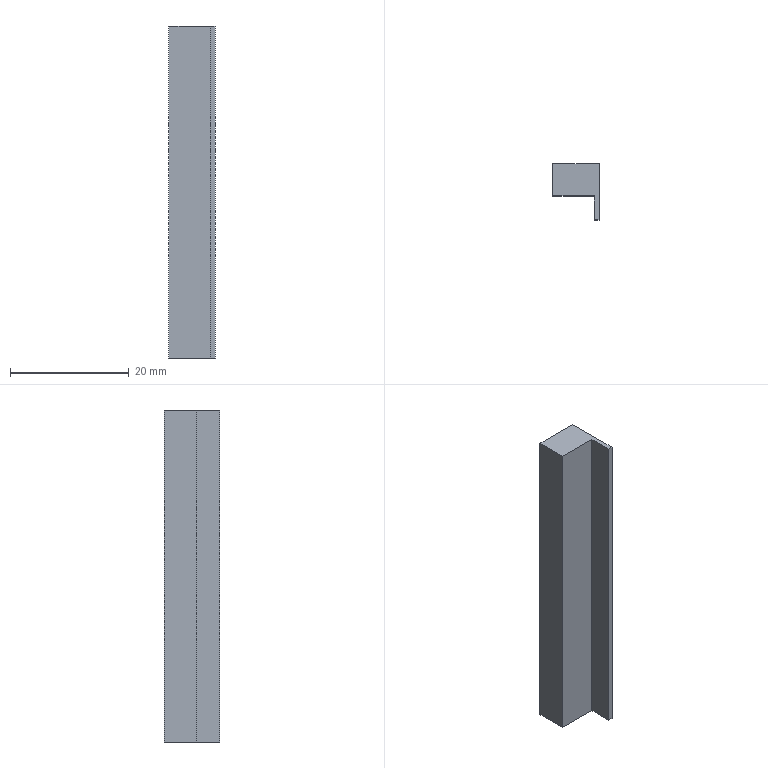Part | NX | features BREP 2 | 2 solids | 16 faces | box 7.8 x 9.398 x 56 mm | volume 5074 mm3 | plane 16
STEP:
#1=CARTESIAN_POINT('',(3.9,4.699,-4.));
#2=VERTEX_POINT('',#1);
#3=CARTESIAN_POINT('',(3.9,4.699,52.));
#4=VERTEX_POINT('',#3);
#5=CARTESIAN_POINT('',(3.9,4.699,0.));
#6=DIRECTION('',(0.,0.,1.));
#7=VECTOR('',#6,1000.);
#8=LINE('',#5,#7);
#9=EDGE_CURVE('',#2,#4,#8,.T.);
#10=ORIENTED_EDGE('',*,*,#9,.T.);
#11=CARTESIAN_POINT('',(3.9,-4.699,52.));
#12=VERTEX_POINT('',#11);
#13=CARTESIAN_POINT('',(3.9,-26.301,52.));
#14=DIRECTION('',(0.,1.,0.));
#15=VECTOR('',#14,1000.);
#16=LINE('',#13,#15);
#17=EDGE_CURVE('',#12,#4,#16,.T.);
#18=ORIENTED_EDGE('',*,*,#17,.F.);
#19=CARTESIAN_POINT('',(3.9,-4.699,-4.));
#20=VERTEX_POINT('',#19);
#21=CARTESIAN_POINT('',(3.9,-4.699,0.));
#22=DIRECTION('',(0.,0.,1.));
#23=VECTOR('',#22,1000.);
#24=LINE('',#21,#23);
#25=EDGE_CURVE('',#20,#12,#24,.T.);
#26=ORIENTED_EDGE('',*,*,#25,.F.);
#27=CARTESIAN_POINT('',(3.9,-26.301,-4.));
#28=DIRECTION('',(0.,1.,0.));
#29=VECTOR('',#28,1000.);
#30=LINE('',#27,#29);
#31=EDGE_CURVE('',#20,#2,#30,.T.);
#32=ORIENTED_EDGE('',*,*,#31,.T.);
#33=EDGE_LOOP('',(#10,#18,#26,#32));
#34=FACE_BOUND('',#33,.T.);
#35=CARTESIAN_POINT('',(3.9,4.699,0.));
#36=DIRECTION('',(-1.,0.,0.));
#37=DIRECTION('',(0.,1.,0.));
#38=AXIS2_PLACEMENT_3D('',#35,#36,#37);
#39=PLANE('',#38);
#40=ADVANCED_FACE('',(#34),#39,.F.);
#41=ORIENTED_EDGE('',*,*,#25,.T.);
#42=CARTESIAN_POINT('',(3.1,-4.699,52.));
#43=VERTEX_POINT('',#42);
#44=CARTESIAN_POINT('',(-9.65,-4.699,52.));
#45=DIRECTION('',(1.,0.,0.));
#46=VECTOR('',#45,1000.);
#47=LINE('',#44,#46);
#48=EDGE_CURVE('',#43,#12,#47,.T.);
#49=ORIENTED_EDGE('',*,*,#48,.F.);
#50=CARTESIAN_POINT('',(3.1,-4.699,-4.));
#51=VERTEX_POINT('',#50);
#52=CARTESIAN_POINT('',(3.1,-4.699,0.));
#53=DIRECTION('',(0.,0.,1.));
#54=VECTOR('',#53,1000.);
#55=LINE('',#52,#54);
#56=EDGE_CURVE('',#51,#43,#55,.T.);
#57=ORIENTED_EDGE('',*,*,#56,.F.);
#58=CARTESIAN_POINT('',(-9.65,-4.699,-4.));
#59=DIRECTION('',(1.,0.,0.));
#60=VECTOR('',#59,1000.);
#61=LINE('',#58,#60);
#62=EDGE_CURVE('',#51,#20,#61,.T.);
#63=ORIENTED_EDGE('',*,*,#62,.T.);
#64=EDGE_LOOP('',(#41,#49,#57,#63));
#65=FACE_BOUND('',#64,.T.);
#66=CARTESIAN_POINT('',(3.9,-4.699,0.));
#67=DIRECTION('',(0.,1.,0.));
#68=DIRECTION('',(1.,0.,0.));
#69=AXIS2_PLACEMENT_3D('',#66,#67,#68);
#70=PLANE('',#69);
#71=ADVANCED_FACE('',(#65),#70,.F.);
#72=ORIENTED_EDGE('',*,*,#56,.T.);
#73=CARTESIAN_POINT('',(3.1,-0.6992,52.));
#74=VERTEX_POINT('',#73);
#75=CARTESIAN_POINT('',(3.1,-26.301,52.));
#76=DIRECTION('',(0.,-1.,0.));
#77=VECTOR('',#76,1000.);
#78=LINE('',#75,#77);
#79=EDGE_CURVE('',#74,#43,#78,.T.);
#80=ORIENTED_EDGE('',*,*,#79,.F.);
#81=CARTESIAN_POINT('',(3.1,-0.6992,-4.));
#82=VERTEX_POINT('',#81);
#83=CARTESIAN_POINT('',(3.1,-0.6992,0.));
#84=DIRECTION('',(0.,0.,1.));
#85=VECTOR('',#84,1000.);
#86=LINE('',#83,#85);
#87=EDGE_CURVE('',#82,#74,#86,.T.);
#88=ORIENTED_EDGE('',*,*,#87,.F.);
#89=CARTESIAN_POINT('',(3.1,-26.301,-4.));
#90=DIRECTION('',(0.,-1.,0.));
#91=VECTOR('',#90,1000.);
#92=LINE('',#89,#91);
#93=EDGE_CURVE('',#82,#51,#92,.T.);
#94=ORIENTED_EDGE('',*,*,#93,.T.);
#95=EDGE_LOOP('',(#72,#80,#88,#94));
#96=FACE_BOUND('',#95,.T.);
#97=CARTESIAN_POINT('',(3.1,-4.699,0.));
#98=DIRECTION('',(1.,0.,0.));
#99=DIRECTION('',(0.,-1.,0.));
#100=AXIS2_PLACEMENT_3D('',#97,#98,#99);
#101=PLANE('',#100);
#102=ADVANCED_FACE('',(#96),#101,.F.);
#103=ORIENTED_EDGE('',*,*,#87,.T.);
#104=CARTESIAN_POINT('',(-3.9,-0.6992,52.));
#105=VERTEX_POINT('',#104);
#106=CARTESIAN_POINT('',(-9.65,-0.6992,52.));
#107=DIRECTION('',(1.,0.,0.));
#108=VECTOR('',#107,1000.);
#109=LINE('',#106,#108);
#110=EDGE_CURVE('',#105,#74,#109,.T.);
#111=ORIENTED_EDGE('',*,*,#110,.F.);
#112=CARTESIAN_POINT('',(-3.9,-0.6992,-4.));
#113=VERTEX_POINT('',#112);
#114=CARTESIAN_POINT('',(-3.9,-0.6992,0.));
#115=DIRECTION('',(0.,0.,1.));
#116=VECTOR('',#115,1000.);
#117=LINE('',#114,#116);
#118=EDGE_CURVE('',#113,#105,#117,.T.);
#119=ORIENTED_EDGE('',*,*,#118,.F.);
#120=CARTESIAN_POINT('',(-9.65,-0.6992,-4.));
#121=DIRECTION('',(1.,0.,0.));
#122=VECTOR('',#121,1000.);
#123=LINE('',#120,#122);
#124=EDGE_CURVE('',#113,#82,#123,.T.);
#125=ORIENTED_EDGE('',*,*,#124,.T.);
#126=EDGE_LOOP('',(#103,#111,#119,#125));
#127=FACE_BOUND('',#126,.T.);
#128=CARTESIAN_POINT('',(3.1,-0.6992,0.));
#129=DIRECTION('',(0.,1.,0.));
#130=DIRECTION('',(1.,0.,0.));
#131=AXIS2_PLACEMENT_3D('',#128,#129,#130);
#132=PLANE('',#131);
#133=ADVANCED_FACE('',(#127),#132,.F.);
#134=CARTESIAN_POINT('',(-3.9,4.699,-4.));
#135=VERTEX_POINT('',#134);
#136=CARTESIAN_POINT('',(-3.9,4.699,52.));
#137=VERTEX_POINT('',#136);
#138=CARTESIAN_POINT('',(-3.9,4.699,0.));
#139=DIRECTION('',(0.,0.,1.));
#140=VECTOR('',#139,1000.);
#141=LINE('',#138,#140);
#142=EDGE_CURVE('',#135,#137,#141,.T.);
#143=ORIENTED_EDGE('',*,*,#142,.F.);
#144=CARTESIAN_POINT('',(-3.9,-26.301,-4.));
#145=DIRECTION('',(0.,-1.,0.));
#146=VECTOR('',#145,1000.);
#147=LINE('',#144,#146);
#148=EDGE_CURVE('',#135,#113,#147,.T.);
#149=ORIENTED_EDGE('',*,*,#148,.T.);
#150=ORIENTED_EDGE('',*,*,#118,.T.);
#151=CARTESIAN_POINT('',(-3.9,-26.301,52.));
#152=DIRECTION('',(0.,-1.,0.));
#153=VECTOR('',#152,1000.);
#154=LINE('',#151,#153);
#155=EDGE_CURVE('',#137,#105,#154,.T.);
#156=ORIENTED_EDGE('',*,*,#155,.F.);
#157=EDGE_LOOP('',(#143,#149,#150,#156));
#158=FACE_BOUND('',#157,.T.);
#159=CARTESIAN_POINT('',(-3.9,2.201,0.));
#160=DIRECTION('',(1.,0.,0.));
#161=DIRECTION('',(0.,-1.,0.));
#162=AXIS2_PLACEMENT_3D('',#159,#160,#161);
#163=PLANE('',#162);
#164=ADVANCED_FACE('',(#158),#163,.F.);
#165=CARTESIAN_POINT('',(-9.65,4.699,-4.));
#166=DIRECTION('',(-1.,0.,0.));
#167=VECTOR('',#166,1000.);
#168=LINE('',#165,#167);
#169=EDGE_CURVE('',#2,#135,#168,.T.);
#170=ORIENTED_EDGE('',*,*,#169,.T.);
#171=ORIENTED_EDGE('',*,*,#142,.T.);
#172=CARTESIAN_POINT('',(-9.65,4.699,52.));
#173=DIRECTION('',(-1.,0.,0.));
#174=VECTOR('',#173,1000.);
#175=LINE('',#172,#174);
#176=EDGE_CURVE('',#4,#137,#175,.T.);
#177=ORIENTED_EDGE('',*,*,#176,.F.);
#178=ORIENTED_EDGE('',*,*,#9,.F.);
#179=EDGE_LOOP('',(#170,#171,#177,#178));
#180=FACE_BOUND('',#179,.T.);
#181=CARTESIAN_POINT('',(-3.9,4.699,0.));
#182=DIRECTION('',(0.,-1.,0.));
#183=DIRECTION('',(-1.,0.,0.));
#184=AXIS2_PLACEMENT_3D('',#181,#182,#183);
#185=PLANE('',#184);
#186=ADVANCED_FACE('',(#180),#185,.F.);
#187=ORIENTED_EDGE('',*,*,#155,.T.);
#188=ORIENTED_EDGE('',*,*,#110,.T.);
#189=ORIENTED_EDGE('',*,*,#79,.T.);
#190=ORIENTED_EDGE('',*,*,#48,.T.);
#191=ORIENTED_EDGE('',*,*,#17,.T.);
#192=ORIENTED_EDGE('',*,*,#176,.T.);
#193=EDGE_LOOP('',(#187,#188,#189,#190,#191,#192));
#194=FACE_BOUND('',#193,.T.);
#195=CARTESIAN_POINT('',(-9.65,-26.301,52.));
#196=DIRECTION('',(0.,0.,1.));
#197=DIRECTION('',(-1.,0.,0.));
#198=AXIS2_PLACEMENT_3D('',#195,#196,#197);
#199=PLANE('',#198);
#200=ADVANCED_FACE('',(#194),#199,.T.);
#201=ORIENTED_EDGE('',*,*,#148,.F.);
#202=ORIENTED_EDGE('',*,*,#169,.F.);
#203=ORIENTED_EDGE('',*,*,#31,.F.);
#204=ORIENTED_EDGE('',*,*,#62,.F.);
#205=ORIENTED_EDGE('',*,*,#93,.F.);
#206=ORIENTED_EDGE('',*,*,#124,.F.);
#207=EDGE_LOOP('',(#201,#202,#203,#204,#205,#206));
#208=FACE_BOUND('',#207,.T.);
#209=CARTESIAN_POINT('',(-9.65,-26.301,-4.));
#210=DIRECTION('',(0.,0.,1.));
#211=DIRECTION('',(-1.,0.,0.));
#212=AXIS2_PLACEMENT_3D('',#209,#210,#211);
#213=PLANE('',#212);
#214=ADVANCED_FACE('',(#208),#213,.F.);
#215=CLOSED_SHELL('',(#40,#71,#102,#133,#164,#186,#200,#214));
#216=MANIFOLD_SOLID_BREP('',#215);
#217=CARTESIAN_POINT('',(3.9,4.699,-4.));
#218=VERTEX_POINT('',#217);
#219=CARTESIAN_POINT('',(3.9,4.699,52.));
#220=VERTEX_POINT('',#219);
#221=CARTESIAN_POINT('',(3.9,4.699,0.));
#222=DIRECTION('',(0.,0.,1.));
#223=VECTOR('',#222,1000.);
#224=LINE('',#221,#223);
#225=EDGE_CURVE('',#218,#220,#224,.T.);
#226=ORIENTED_EDGE('',*,*,#225,.T.);
#227=CARTESIAN_POINT('',(3.9,-4.699,52.));
#228=VERTEX_POINT('',#227);
#229=CARTESIAN_POINT('',(3.9,-26.301,52.));
#230=DIRECTION('',(0.,1.,0.));
#231=VECTOR('',#230,1000.);
#232=LINE('',#229,#231);
#233=EDGE_CURVE('',#228,#220,#232,.T.);
#234=ORIENTED_EDGE('',*,*,#233,.F.);
#235=CARTESIAN_POINT('',(3.9,-4.699,-4.));
#236=VERTEX_POINT('',#235);
#237=CARTESIAN_POINT('',(3.9,-4.699,0.));
#238=DIRECTION('',(0.,0.,1.));
#239=VECTOR('',#238,1000.);
#240=LINE('',#237,#239);
#241=EDGE_CURVE('',#236,#228,#240,.T.);
#242=ORIENTED_EDGE('',*,*,#241,.F.);
#243=CARTESIAN_POINT('',(3.9,-26.301,-4.));
#244=DIRECTION('',(0.,1.,0.));
#245=VECTOR('',#244,1000.);
#246=LINE('',#243,#245);
#247=EDGE_CURVE('',#236,#218,#246,.T.);
#248=ORIENTED_EDGE('',*,*,#247,.T.);
#249=EDGE_LOOP('',(#226,#234,#242,#248));
#250=FACE_BOUND('',#249,.T.);
#251=CARTESIAN_POINT('',(3.9,4.699,0.));
#252=DIRECTION('',(-1.,0.,0.));
#253=DIRECTION('',(0.,1.,0.));
#254=AXIS2_PLACEMENT_3D('',#251,#252,#253);
#255=PLANE('',#254);
#256=ADVANCED_FACE('',(#250),#255,.F.);
#257=ORIENTED_EDGE('',*,*,#241,.T.);
#258=CARTESIAN_POINT('',(3.1,-4.699,52.));
#259=VERTEX_POINT('',#258);
#260=CARTESIAN_POINT('',(-9.65,-4.699,52.));
#261=DIRECTION('',(1.,0.,0.));
#262=VECTOR('',#261,1000.);
#263=LINE('',#260,#262);
#264=EDGE_CURVE('',#259,#228,#263,.T.);
#265=ORIENTED_EDGE('',*,*,#264,.F.);
#266=CARTESIAN_POINT('',(3.1,-4.699,-4.));
#267=VERTEX_POINT('',#266);
#268=CARTESIAN_POINT('',(3.1,-4.699,0.));
#269=DIRECTION('',(0.,0.,1.));
#270=VECTOR('',#269,1000.);
#271=LINE('',#268,#270);
#272=EDGE_CURVE('',#267,#259,#271,.T.);
#273=ORIENTED_EDGE('',*,*,#272,.F.);
#274=CARTESIAN_POINT('',(-9.65,-4.699,-4.));
#275=DIRECTION('',(1.,0.,0.));
#276=VECTOR('',#275,1000.);
#277=LINE('',#274,#276);
#278=EDGE_CURVE('',#267,#236,#277,.T.);
#279=ORIENTED_EDGE('',*,*,#278,.T.);
#280=EDGE_LOOP('',(#257,#265,#273,#279));
#281=FACE_BOUND('',#280,.T.);
#282=CARTESIAN_POINT('',(3.9,-4.699,0.));
#283=DIRECTION('',(0.,1.,0.));
#284=DIRECTION('',(1.,0.,0.));
#285=AXIS2_PLACEMENT_3D('',#282,#283,#284);
#286=PLANE('',#285);
#287=ADVANCED_FACE('',(#281),#286,.F.);
#288=ORIENTED_EDGE('',*,*,#272,.T.);
#289=CARTESIAN_POINT('',(3.1,-0.6992,52.));
#290=VERTEX_POINT('',#289);
#291=CARTESIAN_POINT('',(3.1,-26.301,52.));
#292=DIRECTION('',(0.,-1.,0.));
#293=VECTOR('',#292,1000.);
#294=LINE('',#291,#293);
#295=EDGE_CURVE('',#290,#259,#294,.T.);
#296=ORIENTED_EDGE('',*,*,#295,.F.);
#297=CARTESIAN_POINT('',(3.1,-0.6992,-4.));
#298=VERTEX_POINT('',#297);
#299=CARTESIAN_POINT('',(3.1,-0.6992,0.));
#300=DIRECTION('',(0.,0.,1.));
#301=VECTOR('',#300,1000.);
#302=LINE('',#299,#301);
#303=EDGE_CURVE('',#298,#290,#302,.T.);
#304=ORIENTED_EDGE('',*,*,#303,.F.);
#305=CARTESIAN_POINT('',(3.1,-26.301,-4.));
#306=DIRECTION('',(0.,-1.,0.));
#307=VECTOR('',#306,1000.);
#308=LINE('',#305,#307);
#309=EDGE_CURVE('',#298,#267,#308,.T.);
#310=ORIENTED_EDGE('',*,*,#309,.T.);
#311=EDGE_LOOP('',(#288,#296,#304,#310));
#312=FACE_BOUND('',#311,.T.);
#313=CARTESIAN_POINT('',(3.1,-4.699,0.));
#314=DIRECTION('',(1.,0.,0.));
#315=DIRECTION('',(0.,-1.,0.));
#316=AXIS2_PLACEMENT_3D('',#313,#314,#315);
#317=PLANE('',#316);
#318=ADVANCED_FACE('',(#312),#317,.F.);
#319=ORIENTED_EDGE('',*,*,#303,.T.);
#320=CARTESIAN_POINT('',(-3.9,-0.6992,52.));
#321=VERTEX_POINT('',#320);
#322=CARTESIAN_POINT('',(-9.65,-0.6992,52.));
#323=DIRECTION('',(1.,0.,0.));
#324=VECTOR('',#323,1000.);
#325=LINE('',#322,#324);
#326=EDGE_CURVE('',#321,#290,#325,.T.);
#327=ORIENTED_EDGE('',*,*,#326,.F.);
#328=CARTESIAN_POINT('',(-3.9,-0.6992,-4.));
#329=VERTEX_POINT('',#328);
#330=CARTESIAN_POINT('',(-3.9,-0.6992,0.));
#331=DIRECTION('',(0.,0.,1.));
#332=VECTOR('',#331,1000.);
#333=LINE('',#330,#332);
#334=EDGE_CURVE('',#329,#321,#333,.T.);
#335=ORIENTED_EDGE('',*,*,#334,.F.);
#336=CARTESIAN_POINT('',(-9.65,-0.6992,-4.));
#337=DIRECTION('',(1.,0.,0.));
#338=VECTOR('',#337,1000.);
#339=LINE('',#336,#338);
#340=EDGE_CURVE('',#329,#298,#339,.T.);
#341=ORIENTED_EDGE('',*,*,#340,.T.);
#342=EDGE_LOOP('',(#319,#327,#335,#341));
#343=FACE_BOUND('',#342,.T.);
#344=CARTESIAN_POINT('',(3.1,-0.6992,0.));
#345=DIRECTION('',(0.,1.,0.));
#346=DIRECTION('',(1.,0.,0.));
#347=AXIS2_PLACEMENT_3D('',#344,#345,#346);
#348=PLANE('',#347);
#349=ADVANCED_FACE('',(#343),#348,.F.);
#350=CARTESIAN_POINT('',(-3.9,4.699,-4.));
#351=VERTEX_POINT('',#350);
#352=CARTESIAN_POINT('',(-3.9,4.699,52.));
#353=VERTEX_POINT('',#352);
#354=CARTESIAN_POINT('',(-3.9,4.699,0.));
#355=DIRECTION('',(0.,0.,1.));
#356=VECTOR('',#355,1000.);
#357=LINE('',#354,#356);
#358=EDGE_CURVE('',#351,#353,#357,.T.);
#359=ORIENTED_EDGE('',*,*,#358,.F.);
#360=CARTESIAN_POINT('',(-3.9,-26.301,-4.));
#361=DIRECTION('',(0.,-1.,0.));
#362=VECTOR('',#361,1000.);
#363=LINE('',#360,#362);
#364=EDGE_CURVE('',#351,#329,#363,.T.);
#365=ORIENTED_EDGE('',*,*,#364,.T.);
#366=ORIENTED_EDGE('',*,*,#334,.T.);
#367=CARTESIAN_POINT('',(-3.9,-26.301,52.));
#368=DIRECTION('',(0.,-1.,0.));
#369=VECTOR('',#368,1000.);
#370=LINE('',#367,#369);
#371=EDGE_CURVE('',#353,#321,#370,.T.);
#372=ORIENTED_EDGE('',*,*,#371,.F.);
#373=EDGE_LOOP('',(#359,#365,#366,#372));
#374=FACE_BOUND('',#373,.T.);
#375=CARTESIAN_POINT('',(-3.9,2.201,0.));
#376=DIRECTION('',(1.,0.,0.));
#377=DIRECTION('',(0.,-1.,0.));
#378=AXIS2_PLACEMENT_3D('',#375,#376,#377);
#379=PLANE('',#378);
#380=ADVANCED_FACE('',(#374),#379,.F.);
#381=CARTESIAN_POINT('',(-9.65,4.699,-4.));
#382=DIRECTION('',(-1.,0.,0.));
#383=VECTOR('',#382,1000.);
#384=LINE('',#381,#383);
#385=EDGE_CURVE('',#218,#351,#384,.T.);
#386=ORIENTED_EDGE('',*,*,#385,.T.);
#387=ORIENTED_EDGE('',*,*,#358,.T.);
#388=CARTESIAN_POINT('',(-9.65,4.699,52.));
#389=DIRECTION('',(-1.,0.,0.));
#390=VECTOR('',#389,1000.);
#391=LINE('',#388,#390);
#392=EDGE_CURVE('',#220,#353,#391,.T.);
#393=ORIENTED_EDGE('',*,*,#392,.F.);
#394=ORIENTED_EDGE('',*,*,#225,.F.);
#395=EDGE_LOOP('',(#386,#387,#393,#394));
#396=FACE_BOUND('',#395,.T.);
#397=CARTESIAN_POINT('',(-3.9,4.699,0.));
#398=DIRECTION('',(0.,-1.,0.));
#399=DIRECTION('',(-1.,0.,0.));
#400=AXIS2_PLACEMENT_3D('',#397,#398,#399);
#401=PLANE('',#400);
#402=ADVANCED_FACE('',(#396),#401,.F.);
#403=ORIENTED_EDGE('',*,*,#371,.T.);
#404=ORIENTED_EDGE('',*,*,#326,.T.);
#405=ORIENTED_EDGE('',*,*,#295,.T.);
#406=ORIENTED_EDGE('',*,*,#264,.T.);
#407=ORIENTED_EDGE('',*,*,#233,.T.);
#408=ORIENTED_EDGE('',*,*,#392,.T.);
#409=EDGE_LOOP('',(#403,#404,#405,#406,#407,#408));
#410=FACE_BOUND('',#409,.T.);
#411=CARTESIAN_POINT('',(-9.65,-26.301,52.));
#412=DIRECTION('',(0.,0.,1.));
#413=DIRECTION('',(-1.,0.,0.));
#414=AXIS2_PLACEMENT_3D('',#411,#412,#413);
#415=PLANE('',#414);
#416=ADVANCED_FACE('',(#410),#415,.T.);
#417=ORIENTED_EDGE('',*,*,#364,.F.);
#418=ORIENTED_EDGE('',*,*,#385,.F.);
#419=ORIENTED_EDGE('',*,*,#247,.F.);
#420=ORIENTED_EDGE('',*,*,#278,.F.);
#421=ORIENTED_EDGE('',*,*,#309,.F.);
#422=ORIENTED_EDGE('',*,*,#340,.F.);
#423=EDGE_LOOP('',(#417,#418,#419,#420,#421,#422));
#424=FACE_BOUND('',#423,.T.);
#425=CARTESIAN_POINT('',(-9.65,-26.301,-4.));
#426=DIRECTION('',(0.,0.,1.));
#427=DIRECTION('',(-1.,0.,0.));
#428=AXIS2_PLACEMENT_3D('',#425,#426,#427);
#429=PLANE('',#428);
#430=ADVANCED_FACE('',(#424),#429,.F.);
#431=CLOSED_SHELL('',(#256,#287,#318,#349,#380,#402,#416,#430));
#432=MANIFOLD_SOLID_BREP('',#431);
#433=(LENGTH_UNIT()NAMED_UNIT(*)SI_UNIT(.MILLI.,.METRE.));
#434=UNCERTAINTY_MEASURE_WITH_UNIT(LENGTH_MEASURE(0.00001),#433,'','');
#435=(NAMED_UNIT(*)PLANE_ANGLE_UNIT()SI_UNIT($,.RADIAN.));
#436=(NAMED_UNIT(*)SI_UNIT($,.STERADIAN.)SOLID_ANGLE_UNIT());
#437=(GEOMETRIC_REPRESENTATION_CONTEXT(3)GLOBAL_UNCERTAINTY_ASSIGNED_CONTEXT((#434))GLOBAL_UNIT_ASSIGNED_CONTEXT((#433,#435,#436))REPRESENTATION_CONTEXT('',''));
#438=ADVANCED_BREP_SHAPE_REPRESENTATION('',(#216,#432),#437);